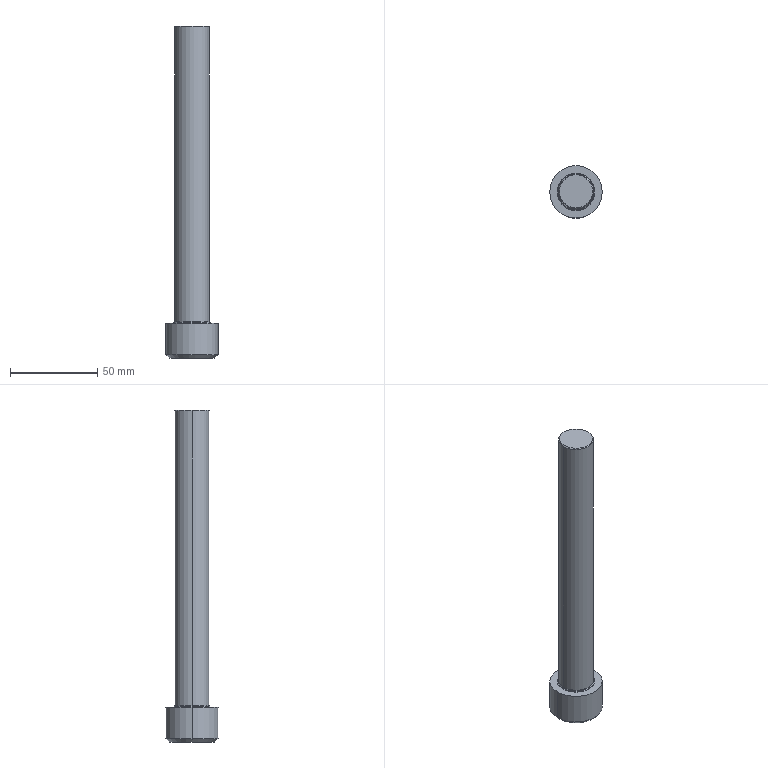Part | Creo | 1 solid | 23 faces | box 30 x 30 x 190 mm | volume 64306 mm3 | plane 9 | cone 6 | cylinder 4 | torus 4 | commonest cylinder face diameters 20 x2 30 x2
STEP:
#1=CARTESIAN_POINT('',(-224.815,189.995,-354.));
#2=VERTEX_POINT('',#1);
#3=CARTESIAN_POINT('',(-219.907,198.495,-354.));
#4=VERTEX_POINT('',#3);
#5=CARTESIAN_POINT('',(-224.815,189.995,-354.));
#6=CARTESIAN_POINT('',(-224.548,190.458,-353.846));
#7=CARTESIAN_POINT('',(-224.012,191.386,-353.574));
#8=CARTESIAN_POINT('',(-223.192,192.806,-353.304));
#9=CARTESIAN_POINT('',(-222.364,194.241,-353.209));
#10=CARTESIAN_POINT('',(-221.532,195.681,-353.304));
#11=CARTESIAN_POINT('',(-220.714,197.099,-353.572));
#12=CARTESIAN_POINT('',(-220.176,198.031,-353.845));
#13=CARTESIAN_POINT('',(-219.907,198.495,-354.));
#14=B_SPLINE_CURVE_WITH_KNOTS('',3,(#5,#6,#7,#8,#9,#10,#11,#12,#13),.UNSPECIFIED.,.F.,.F.,(4,1,1,1,1,1,4),(0.,0.1667,0.3333,0.5,0.6667,0.8333,1.),.UNSPECIFIED.);
#15=EDGE_CURVE('',#2,#4,#14,.T.);
#16=ORIENTED_EDGE('',*,*,#15,.F.);
#17=CARTESIAN_POINT('',(-215.,189.995,-348.333));
#18=VERTEX_POINT('',#17);
#19=CARTESIAN_POINT('',(-215.,189.995,-348.333));
#20=DIRECTION('',(-0.866,0.,-0.5));
#21=VECTOR('',#20,11.333);
#22=LINE('',#19,#21);
#23=EDGE_CURVE('',#18,#2,#22,.T.);
#24=ORIENTED_EDGE('',*,*,#23,.F.);
#25=CARTESIAN_POINT('',(-205.185,189.995,-354.));
#26=VERTEX_POINT('',#25);
#27=CARTESIAN_POINT('',(-215.,189.995,-348.333));
#28=DIRECTION('',(0.866,0.,-0.5));
#29=VECTOR('',#28,11.333);
#30=LINE('',#27,#29);
#31=EDGE_CURVE('',#18,#26,#30,.T.);
#32=ORIENTED_EDGE('',*,*,#31,.T.);
#33=CARTESIAN_POINT('',(-210.093,198.495,-354.));
#34=VERTEX_POINT('',#33);
#35=CARTESIAN_POINT('',(-210.093,198.495,-354.));
#36=CARTESIAN_POINT('',(-209.826,198.033,-353.846));
#37=CARTESIAN_POINT('',(-209.29,197.104,-353.574));
#38=CARTESIAN_POINT('',(-208.47,195.684,-353.304));
#39=CARTESIAN_POINT('',(-207.641,194.25,-353.209));
#40=CARTESIAN_POINT('',(-206.81,192.809,-353.304));
#41=CARTESIAN_POINT('',(-205.991,191.391,-353.572));
#42=CARTESIAN_POINT('',(-205.453,190.46,-353.845));
#43=CARTESIAN_POINT('',(-205.185,189.995,-354.));
#44=B_SPLINE_CURVE_WITH_KNOTS('',3,(#35,#36,#37,#38,#39,#40,#41,#42,#43),.UNSPECIFIED.,.F.,.F.,(4,1,1,1,1,1,4),(0.,0.1667,0.3333,0.5,0.6667,0.8333,1.),.UNSPECIFIED.);
#45=EDGE_CURVE('',#34,#26,#44,.T.);
#46=ORIENTED_EDGE('',*,*,#45,.F.);
#47=CARTESIAN_POINT('',(-219.907,198.495,-354.));
#48=CARTESIAN_POINT('',(-219.376,198.495,-353.847));
#49=CARTESIAN_POINT('',(-218.307,198.495,-353.575));
#50=CARTESIAN_POINT('',(-216.662,198.495,-353.304));
#51=CARTESIAN_POINT('',(-215.002,198.495,-353.209));
#52=CARTESIAN_POINT('',(-213.345,198.495,-353.303));
#53=CARTESIAN_POINT('',(-211.701,198.495,-353.573));
#54=CARTESIAN_POINT('',(-210.627,198.495,-353.846));
#55=CARTESIAN_POINT('',(-210.093,198.495,-354.));
#56=B_SPLINE_CURVE_WITH_KNOTS('',3,(#47,#48,#49,#50,#51,#52,#53,#54,#55),.UNSPECIFIED.,.F.,.F.,(4,1,1,1,1,1,4),(0.,0.1667,0.3333,0.5,0.6667,0.8333,1.),.UNSPECIFIED.);
#57=EDGE_CURVE('',#4,#34,#56,.T.);
#58=ORIENTED_EDGE('',*,*,#57,.F.);
#59=EDGE_LOOP('',(#16,#24,#32,#46,#58));
#60=FACE_OUTER_BOUND('',#59,.F.);
#61=CARTESIAN_POINT('',(-215.,189.995,-351.225));
#62=DIRECTION('',(0.,0.,-1.));
#63=DIRECTION('',(-1.,0.,0.));
#64=AXIS2_PLACEMENT_3D('',#61,#62,#63);
#65=CONICAL_SURFACE('',#64,5.009,60.);
#66=ADVANCED_FACE('',(#60),#65,.F.);
#67=CARTESIAN_POINT('',(-219.907,198.495,-364.));
#68=VERTEX_POINT('',#67);
#69=CARTESIAN_POINT('',(-224.815,189.995,-364.));
#70=VERTEX_POINT('',#69);
#71=CARTESIAN_POINT('',(-219.907,198.495,-364.));
#72=DIRECTION('',(-0.5,-0.866,0.));
#73=VECTOR('',#72,9.815);
#74=LINE('',#71,#73);
#75=EDGE_CURVE('',#68,#70,#74,.T.);
#76=ORIENTED_EDGE('',*,*,#75,.T.);
#77=CARTESIAN_POINT('',(-224.815,189.995,-364.));
#78=DIRECTION('',(0.,0.,1.));
#79=VECTOR('',#78,10.);
#80=LINE('',#77,#79);
#81=EDGE_CURVE('',#70,#2,#80,.T.);
#82=ORIENTED_EDGE('',*,*,#81,.T.);
#83=ORIENTED_EDGE('',*,*,#15,.T.);
#84=CARTESIAN_POINT('',(-219.907,198.495,-364.));
#85=DIRECTION('',(0.,0.,1.));
#86=VECTOR('',#85,10.);
#87=LINE('',#84,#86);
#88=EDGE_CURVE('',#68,#4,#87,.T.);
#89=ORIENTED_EDGE('',*,*,#88,.F.);
#90=EDGE_LOOP('',(#76,#82,#83,#89));
#91=FACE_OUTER_BOUND('',#90,.F.);
#92=CARTESIAN_POINT('',(-219.907,198.495,-354.));
#93=DIRECTION('',(0.866,-0.5,0.));
#94=DIRECTION('',(-0.5,-0.866,0.));
#95=AXIS2_PLACEMENT_3D('',#92,#93,#94);
#96=PLANE('',#95);
#97=ADVANCED_FACE('',(#91),#96,.T.);
#98=CARTESIAN_POINT('',(-228.,189.995,-364.));
#99=VERTEX_POINT('',#98);
#100=CARTESIAN_POINT('',(-202.,189.995,-364.));
#101=VERTEX_POINT('',#100);
#102=CARTESIAN_POINT('',(-215.,189.995,-364.));
#103=DIRECTION('',(0.,0.,-1.));
#104=DIRECTION('',(-1.,0.,0.));
#105=AXIS2_PLACEMENT_3D('',#102,#103,#104);
#106=CIRCLE('',#105,13.);
#107=EDGE_CURVE('',#99,#101,#106,.T.);
#108=ORIENTED_EDGE('',*,*,#107,.F.);
#109=CARTESIAN_POINT('',(-215.,189.995,-364.));
#110=DIRECTION('',(0.,0.,-1.));
#111=DIRECTION('',(1.,0.,0.));
#112=AXIS2_PLACEMENT_3D('',#109,#110,#111);
#113=CIRCLE('',#112,13.);
#114=EDGE_CURVE('',#101,#99,#113,.T.);
#115=ORIENTED_EDGE('',*,*,#114,.F.);
#116=EDGE_LOOP('',(#108,#115));
#117=FACE_OUTER_BOUND('',#116,.F.);
#118=CARTESIAN_POINT('',(-219.907,181.495,-364.));
#119=VERTEX_POINT('',#118);
#120=CARTESIAN_POINT('',(-224.815,189.995,-364.));
#121=DIRECTION('',(0.5,-0.866,0.));
#122=VECTOR('',#121,9.815);
#123=LINE('',#120,#122);
#124=EDGE_CURVE('',#70,#119,#123,.T.);
#125=ORIENTED_EDGE('',*,*,#124,.F.);
#126=ORIENTED_EDGE('',*,*,#75,.F.);
#127=CARTESIAN_POINT('',(-210.093,198.495,-364.));
#128=VERTEX_POINT('',#127);
#129=CARTESIAN_POINT('',(-219.907,198.495,-364.));
#130=DIRECTION('',(1.,0.,0.));
#131=VECTOR('',#130,9.815);
#132=LINE('',#129,#131);
#133=EDGE_CURVE('',#68,#128,#132,.T.);
#134=ORIENTED_EDGE('',*,*,#133,.T.);
#135=CARTESIAN_POINT('',(-205.185,189.995,-364.));
#136=VERTEX_POINT('',#135);
#137=CARTESIAN_POINT('',(-205.185,189.995,-364.));
#138=DIRECTION('',(-0.5,0.866,0.));
#139=VECTOR('',#138,9.815);
#140=LINE('',#137,#139);
#141=EDGE_CURVE('',#136,#128,#140,.T.);
#142=ORIENTED_EDGE('',*,*,#141,.F.);
#143=CARTESIAN_POINT('',(-210.093,181.495,-364.));
#144=VERTEX_POINT('',#143);
#145=CARTESIAN_POINT('',(-210.093,181.495,-364.));
#146=DIRECTION('',(0.5,0.866,0.));
#147=VECTOR('',#146,9.815);
#148=LINE('',#145,#147);
#149=EDGE_CURVE('',#144,#136,#148,.T.);
#150=ORIENTED_EDGE('',*,*,#149,.F.);
#151=CARTESIAN_POINT('',(-210.093,181.495,-364.));
#152=DIRECTION('',(-1.,0.,0.));
#153=VECTOR('',#152,9.815);
#154=LINE('',#151,#153);
#155=EDGE_CURVE('',#144,#119,#154,.T.);
#156=ORIENTED_EDGE('',*,*,#155,.T.);
#157=EDGE_LOOP('',(#125,#126,#134,#142,#150,#156));
#158=FACE_BOUND('',#157,.F.);
#159=CARTESIAN_POINT('',(-215.,189.995,-364.));
#160=DIRECTION('',(0.,0.,-1.));
#161=DIRECTION('',(-1.,0.,0.));
#162=AXIS2_PLACEMENT_3D('',#159,#160,#161);
#163=PLANE('',#162);
#164=ADVANCED_FACE('',(#117,#158),#163,.T.);
#165=CARTESIAN_POINT('',(-230.,189.995,-362.));
#166=VERTEX_POINT('',#165);
#167=CARTESIAN_POINT('',(-200.,189.995,-362.));
#168=VERTEX_POINT('',#167);
#169=CARTESIAN_POINT('',(-215.,189.995,-362.));
#170=DIRECTION('',(0.,0.,-1.));
#171=DIRECTION('',(-1.,0.,0.));
#172=AXIS2_PLACEMENT_3D('',#169,#170,#171);
#173=CIRCLE('',#172,15.);
#174=EDGE_CURVE('',#166,#168,#173,.T.);
#175=ORIENTED_EDGE('',*,*,#174,.F.);
#176=CARTESIAN_POINT('',(-228.,189.995,-364.));
#177=DIRECTION('',(-0.7071,0.,0.7071));
#178=VECTOR('',#177,2.828);
#179=LINE('',#176,#178);
#180=EDGE_CURVE('',#99,#166,#179,.T.);
#181=ORIENTED_EDGE('',*,*,#180,.F.);
#182=ORIENTED_EDGE('',*,*,#107,.T.);
#183=CARTESIAN_POINT('',(-202.,189.995,-364.));
#184=DIRECTION('',(0.7071,0.,0.7071));
#185=VECTOR('',#184,2.828);
#186=LINE('',#183,#185);
#187=EDGE_CURVE('',#101,#168,#186,.T.);
#188=ORIENTED_EDGE('',*,*,#187,.T.);
#189=EDGE_LOOP('',(#175,#181,#182,#188));
#190=FACE_OUTER_BOUND('',#189,.F.);
#191=CARTESIAN_POINT('',(-215.,189.995,-363.));
#192=DIRECTION('',(0.,0.,1.));
#193=DIRECTION('',(1.,0.,0.));
#194=AXIS2_PLACEMENT_3D('',#191,#192,#193);
#195=CONICAL_SURFACE('',#194,14.,45.);
#196=ADVANCED_FACE('',(#190),#195,.T.);
#197=ORIENTED_EDGE('',*,*,#174,.T.);
#198=CARTESIAN_POINT('',(-200.,189.995,-344.));
#199=VERTEX_POINT('',#198);
#200=CARTESIAN_POINT('',(-200.,189.995,-344.));
#201=DIRECTION('',(0.,0.,-1.));
#202=VECTOR('',#201,18.);
#203=LINE('',#200,#202);
#204=EDGE_CURVE('',#199,#168,#203,.T.);
#205=ORIENTED_EDGE('',*,*,#204,.F.);
#206=CARTESIAN_POINT('',(-230.,189.995,-344.));
#207=VERTEX_POINT('',#206);
#208=CARTESIAN_POINT('',(-215.,189.995,-344.));
#209=DIRECTION('',(0.,0.,1.));
#210=DIRECTION('',(1.,0.,0.));
#211=AXIS2_PLACEMENT_3D('',#208,#209,#210);
#212=CIRCLE('',#211,15.);
#213=EDGE_CURVE('',#199,#207,#212,.T.);
#214=ORIENTED_EDGE('',*,*,#213,.T.);
#215=CARTESIAN_POINT('',(-230.,189.995,-344.));
#216=DIRECTION('',(0.,0.,-1.));
#217=VECTOR('',#216,18.);
#218=LINE('',#215,#217);
#219=EDGE_CURVE('',#207,#166,#218,.T.);
#220=ORIENTED_EDGE('',*,*,#219,.T.);
#221=EDGE_LOOP('',(#197,#205,#214,#220));
#222=FACE_OUTER_BOUND('',#221,.F.);
#223=CARTESIAN_POINT('',(-215.,189.995,-344.));
#224=DIRECTION('',(0.,0.,-1.));
#225=DIRECTION('',(-1.,0.,0.));
#226=AXIS2_PLACEMENT_3D('',#223,#224,#225);
#227=CYLINDRICAL_SURFACE('',#226,15.);
#228=ADVANCED_FACE('',(#222),#227,.T.);
#229=CARTESIAN_POINT('',(-215.,189.995,-362.));
#230=DIRECTION('',(0.,0.,-1.));
#231=DIRECTION('',(1.,0.,0.));
#232=AXIS2_PLACEMENT_3D('',#229,#230,#231);
#233=CIRCLE('',#232,15.);
#234=EDGE_CURVE('',#168,#166,#233,.T.);
#235=ORIENTED_EDGE('',*,*,#234,.T.);
#236=ORIENTED_EDGE('',*,*,#219,.F.);
#237=CARTESIAN_POINT('',(-215.,189.995,-344.));
#238=DIRECTION('',(0.,0.,1.));
#239=DIRECTION('',(-1.,0.,0.));
#240=AXIS2_PLACEMENT_3D('',#237,#238,#239);
#241=CIRCLE('',#240,15.);
#242=EDGE_CURVE('',#207,#199,#241,.T.);
#243=ORIENTED_EDGE('',*,*,#242,.T.);
#244=ORIENTED_EDGE('',*,*,#204,.T.);
#245=EDGE_LOOP('',(#235,#236,#243,#244));
#246=FACE_OUTER_BOUND('',#245,.F.);
#247=CARTESIAN_POINT('',(-215.,189.995,-344.));
#248=DIRECTION('',(0.,0.,-1.));
#249=DIRECTION('',(-1.,0.,0.));
#250=AXIS2_PLACEMENT_3D('',#247,#248,#249);
#251=CYLINDRICAL_SURFACE('',#250,15.);
#252=ADVANCED_FACE('',(#246),#251,.T.);
#253=ORIENTED_EDGE('',*,*,#234,.F.);
#254=ORIENTED_EDGE('',*,*,#187,.F.);
#255=ORIENTED_EDGE('',*,*,#114,.T.);
#256=ORIENTED_EDGE('',*,*,#180,.T.);
#257=EDGE_LOOP('',(#253,#254,#255,#256));
#258=FACE_OUTER_BOUND('',#257,.F.);
#259=CARTESIAN_POINT('',(-215.,189.995,-363.));
#260=DIRECTION('',(0.,0.,1.));
#261=DIRECTION('',(1.,0.,0.));
#262=AXIS2_PLACEMENT_3D('',#259,#260,#261);
#263=CONICAL_SURFACE('',#262,14.,45.);
#264=ADVANCED_FACE('',(#258),#263,.T.);
#265=ORIENTED_EDGE('',*,*,#242,.F.);
#266=ORIENTED_EDGE('',*,*,#213,.F.);
#267=EDGE_LOOP('',(#265,#266));
#268=FACE_OUTER_BOUND('',#267,.F.);
#269=CARTESIAN_POINT('',(-225.8,189.995,-344.));
#270=VERTEX_POINT('',#269);
#271=CARTESIAN_POINT('',(-204.2,189.995,-344.));
#272=VERTEX_POINT('',#271);
#273=CARTESIAN_POINT('',(-215.,189.995,-344.));
#274=DIRECTION('',(0.,0.,-1.));
#275=DIRECTION('',(-1.,0.,0.));
#276=AXIS2_PLACEMENT_3D('',#273,#274,#275);
#277=CIRCLE('',#276,10.8);
#278=EDGE_CURVE('',#270,#272,#277,.T.);
#279=ORIENTED_EDGE('',*,*,#278,.F.);
#280=CARTESIAN_POINT('',(-215.,189.995,-344.));
#281=DIRECTION('',(0.,0.,-1.));
#282=DIRECTION('',(1.,0.,0.));
#283=AXIS2_PLACEMENT_3D('',#280,#281,#282);
#284=CIRCLE('',#283,10.8);
#285=EDGE_CURVE('',#272,#270,#284,.T.);
#286=ORIENTED_EDGE('',*,*,#285,.F.);
#287=EDGE_LOOP('',(#279,#286));
#288=FACE_BOUND('',#287,.F.);
#289=CARTESIAN_POINT('',(-215.,189.995,-344.));
#290=DIRECTION('',(0.,0.,-1.));
#291=DIRECTION('',(-1.,0.,0.));
#292=AXIS2_PLACEMENT_3D('',#289,#290,#291);
#293=PLANE('',#292);
#294=ADVANCED_FACE('',(#268,#288),#293,.F.);
#295=ORIENTED_EDGE('',*,*,#278,.T.);
#296=CARTESIAN_POINT('',(-204.766,189.995,-343.766));
#297=VERTEX_POINT('',#296);
#298=CARTESIAN_POINT('',(-204.2,189.995,-343.2));
#299=DIRECTION('',(0.,1.,0.));
#300=DIRECTION('',(0.,0.,-1.));
#301=AXIS2_PLACEMENT_3D('',#298,#299,#300);
#302=CIRCLE('',#301,0.8);
#303=EDGE_CURVE('',#272,#297,#302,.T.);
#304=ORIENTED_EDGE('',*,*,#303,.T.);
#305=CARTESIAN_POINT('',(-225.234,189.995,-343.766));
#306=VERTEX_POINT('',#305);
#307=CARTESIAN_POINT('',(-215.,189.995,-343.766));
#308=DIRECTION('',(0.,0.,-1.));
#309=DIRECTION('',(-1.,0.,0.));
#310=AXIS2_PLACEMENT_3D('',#307,#308,#309);
#311=CIRCLE('',#310,10.234);
#312=EDGE_CURVE('',#306,#297,#311,.T.);
#313=ORIENTED_EDGE('',*,*,#312,.F.);
#314=CARTESIAN_POINT('',(-225.8,189.995,-343.2));
#315=DIRECTION('',(0.,-1.,0.));
#316=DIRECTION('',(0.,0.,-1.));
#317=AXIS2_PLACEMENT_3D('',#314,#315,#316);
#318=CIRCLE('',#317,0.8);
#319=EDGE_CURVE('',#270,#306,#318,.T.);
#320=ORIENTED_EDGE('',*,*,#319,.F.);
#321=EDGE_LOOP('',(#295,#304,#313,#320));
#322=FACE_OUTER_BOUND('',#321,.F.);
#323=CARTESIAN_POINT('',(-215.,189.995,-343.2));
#324=DIRECTION('',(0.,0.,-1.));
#325=DIRECTION('',(-1.,0.,0.));
#326=AXIS2_PLACEMENT_3D('',#323,#324,#325);
#327=TOROIDAL_SURFACE('',#326,10.8,0.8);
#328=ADVANCED_FACE('',(#322),#327,.F.);
#329=ORIENTED_EDGE('',*,*,#285,.T.);
#330=ORIENTED_EDGE('',*,*,#319,.T.);
#331=CARTESIAN_POINT('',(-215.,189.995,-343.766));
#332=DIRECTION('',(0.,0.,-1.));
#333=DIRECTION('',(1.,0.,0.));
#334=AXIS2_PLACEMENT_3D('',#331,#332,#333);
#335=CIRCLE('',#334,10.234);
#336=EDGE_CURVE('',#297,#306,#335,.T.);
#337=ORIENTED_EDGE('',*,*,#336,.F.);
#338=ORIENTED_EDGE('',*,*,#303,.F.);
#339=EDGE_LOOP('',(#329,#330,#337,#338));
#340=FACE_OUTER_BOUND('',#339,.F.);
#341=CARTESIAN_POINT('',(-215.,189.995,-343.2));
#342=DIRECTION('',(0.,0.,-1.));
#343=DIRECTION('',(-1.,0.,0.));
#344=AXIS2_PLACEMENT_3D('',#341,#342,#343);
#345=TOROIDAL_SURFACE('',#344,10.8,0.8);
#346=ADVANCED_FACE('',(#340),#345,.F.);
#347=CARTESIAN_POINT('',(-205.,189.995,-343.2));
#348=VERTEX_POINT('',#347);
#349=CARTESIAN_POINT('',(-225.,189.995,-343.2));
#350=VERTEX_POINT('',#349);
#351=CARTESIAN_POINT('',(-215.,189.995,-343.2));
#352=DIRECTION('',(0.,0.,-1.));
#353=DIRECTION('',(1.,0.,0.));
#354=AXIS2_PLACEMENT_3D('',#351,#352,#353);
#355=CIRCLE('',#354,10.);
#356=EDGE_CURVE('',#348,#350,#355,.T.);
#357=ORIENTED_EDGE('',*,*,#356,.F.);
#358=CARTESIAN_POINT('',(-204.2,189.995,-343.2));
#359=DIRECTION('',(0.,1.,0.));
#360=DIRECTION('',(-0.7071,0.,-0.7071));
#361=AXIS2_PLACEMENT_3D('',#358,#359,#360);
#362=CIRCLE('',#361,0.8);
#363=EDGE_CURVE('',#297,#348,#362,.T.);
#364=ORIENTED_EDGE('',*,*,#363,.F.);
#365=ORIENTED_EDGE('',*,*,#336,.T.);
#366=CARTESIAN_POINT('',(-225.8,189.995,-343.2));
#367=DIRECTION('',(0.,-1.,0.));
#368=DIRECTION('',(0.7071,0.,-0.7071));
#369=AXIS2_PLACEMENT_3D('',#366,#367,#368);
#370=CIRCLE('',#369,0.8);
#371=EDGE_CURVE('',#306,#350,#370,.T.);
#372=ORIENTED_EDGE('',*,*,#371,.T.);
#373=EDGE_LOOP('',(#357,#364,#365,#372));
#374=FACE_OUTER_BOUND('',#373,.F.);
#375=CARTESIAN_POINT('',(-215.,189.995,-343.2));
#376=DIRECTION('',(0.,0.,-1.));
#377=DIRECTION('',(-1.,0.,0.));
#378=AXIS2_PLACEMENT_3D('',#375,#376,#377);
#379=TOROIDAL_SURFACE('',#378,10.8,0.8);
#380=ADVANCED_FACE('',(#374),#379,.F.);
#381=CARTESIAN_POINT('',(-225.,189.995,-174.5));
#382=VERTEX_POINT('',#381);
#383=CARTESIAN_POINT('',(-205.,189.995,-174.5));
#384=VERTEX_POINT('',#383);
#385=CARTESIAN_POINT('',(-215.,189.995,-174.5));
#386=DIRECTION('',(0.,0.,1.));
#387=DIRECTION('',(-1.,0.,0.));
#388=AXIS2_PLACEMENT_3D('',#385,#386,#387);
#389=CIRCLE('',#388,10.);
#390=EDGE_CURVE('',#382,#384,#389,.T.);
#391=ORIENTED_EDGE('',*,*,#390,.T.);
#392=CARTESIAN_POINT('',(-205.,189.995,-174.5));
#393=DIRECTION('',(0.,0.,-1.));
#394=VECTOR('',#393,168.7);
#395=LINE('',#392,#394);
#396=EDGE_CURVE('',#384,#348,#395,.T.);
#397=ORIENTED_EDGE('',*,*,#396,.T.);
#398=ORIENTED_EDGE('',*,*,#356,.T.);
#399=CARTESIAN_POINT('',(-225.,189.995,-174.5));
#400=DIRECTION('',(0.,0.,-1.));
#401=VECTOR('',#400,168.7);
#402=LINE('',#399,#401);
#403=EDGE_CURVE('',#382,#350,#402,.T.);
#404=ORIENTED_EDGE('',*,*,#403,.F.);
#405=EDGE_LOOP('',(#391,#397,#398,#404));
#406=FACE_OUTER_BOUND('',#405,.F.);
#407=CARTESIAN_POINT('',(-215.,189.995,-174.));
#408=DIRECTION('',(0.,0.,-1.));
#409=DIRECTION('',(-1.,0.,0.));
#410=AXIS2_PLACEMENT_3D('',#407,#408,#409);
#411=CYLINDRICAL_SURFACE('',#410,10.);
#412=ADVANCED_FACE('',(#406),#411,.T.);
#413=CARTESIAN_POINT('',(-224.5,189.995,-174.));
#414=VERTEX_POINT('',#413);
#415=CARTESIAN_POINT('',(-205.5,189.995,-174.));
#416=VERTEX_POINT('',#415);
#417=CARTESIAN_POINT('',(-215.,189.995,-174.));
#418=DIRECTION('',(0.,0.,1.));
#419=DIRECTION('',(-1.,0.,0.));
#420=AXIS2_PLACEMENT_3D('',#417,#418,#419);
#421=CIRCLE('',#420,9.5);
#422=EDGE_CURVE('',#414,#416,#421,.T.);
#423=ORIENTED_EDGE('',*,*,#422,.T.);
#424=CARTESIAN_POINT('',(-205.5,189.995,-174.));
#425=DIRECTION('',(0.7071,0.,-0.7071));
#426=VECTOR('',#425,0.7071);
#427=LINE('',#424,#426);
#428=EDGE_CURVE('',#416,#384,#427,.T.);
#429=ORIENTED_EDGE('',*,*,#428,.T.);
#430=ORIENTED_EDGE('',*,*,#390,.F.);
#431=CARTESIAN_POINT('',(-224.5,189.995,-174.));
#432=DIRECTION('',(-0.7071,0.,-0.7071));
#433=VECTOR('',#432,0.7071);
#434=LINE('',#431,#433);
#435=EDGE_CURVE('',#414,#382,#434,.T.);
#436=ORIENTED_EDGE('',*,*,#435,.F.);
#437=EDGE_LOOP('',(#423,#429,#430,#436));
#438=FACE_OUTER_BOUND('',#437,.F.);
#439=CARTESIAN_POINT('',(-215.,189.995,-174.25));
#440=DIRECTION('',(0.,0.,-1.));
#441=DIRECTION('',(-1.,0.,0.));
#442=AXIS2_PLACEMENT_3D('',#439,#440,#441);
#443=CONICAL_SURFACE('',#442,9.75,45.);
#444=ADVANCED_FACE('',(#438),#443,.T.);
#445=ORIENTED_EDGE('',*,*,#422,.F.);
#446=CARTESIAN_POINT('',(-215.,189.995,-174.));
#447=DIRECTION('',(0.,0.,1.));
#448=DIRECTION('',(1.,0.,0.));
#449=AXIS2_PLACEMENT_3D('',#446,#447,#448);
#450=CIRCLE('',#449,9.5);
#451=EDGE_CURVE('',#416,#414,#450,.T.);
#452=ORIENTED_EDGE('',*,*,#451,.F.);
#453=EDGE_LOOP('',(#445,#452));
#454=FACE_OUTER_BOUND('',#453,.F.);
#455=CARTESIAN_POINT('',(-215.,189.995,-174.));
#456=DIRECTION('',(0.,0.,-1.));
#457=DIRECTION('',(-1.,0.,0.));
#458=AXIS2_PLACEMENT_3D('',#455,#456,#457);
#459=PLANE('',#458);
#460=ADVANCED_FACE('',(#454),#459,.F.);
#461=ORIENTED_EDGE('',*,*,#451,.T.);
#462=ORIENTED_EDGE('',*,*,#435,.T.);
#463=CARTESIAN_POINT('',(-215.,189.995,-174.5));
#464=DIRECTION('',(0.,0.,1.));
#465=DIRECTION('',(1.,0.,0.));
#466=AXIS2_PLACEMENT_3D('',#463,#464,#465);
#467=CIRCLE('',#466,10.);
#468=EDGE_CURVE('',#384,#382,#467,.T.);
#469=ORIENTED_EDGE('',*,*,#468,.F.);
#470=ORIENTED_EDGE('',*,*,#428,.F.);
#471=EDGE_LOOP('',(#461,#462,#469,#470));
#472=FACE_OUTER_BOUND('',#471,.F.);
#473=CARTESIAN_POINT('',(-215.,189.995,-174.25));
#474=DIRECTION('',(0.,0.,-1.));
#475=DIRECTION('',(-1.,0.,0.));
#476=AXIS2_PLACEMENT_3D('',#473,#474,#475);
#477=CONICAL_SURFACE('',#476,9.75,45.);
#478=ADVANCED_FACE('',(#472),#477,.T.);
#479=ORIENTED_EDGE('',*,*,#468,.T.);
#480=ORIENTED_EDGE('',*,*,#403,.T.);
#481=CARTESIAN_POINT('',(-215.,189.995,-343.2));
#482=DIRECTION('',(0.,0.,-1.));
#483=DIRECTION('',(-1.,0.,0.));
#484=AXIS2_PLACEMENT_3D('',#481,#482,#483);
#485=CIRCLE('',#484,10.);
#486=EDGE_CURVE('',#350,#348,#485,.T.);
#487=ORIENTED_EDGE('',*,*,#486,.T.);
#488=ORIENTED_EDGE('',*,*,#396,.F.);
#489=EDGE_LOOP('',(#479,#480,#487,#488));
#490=FACE_OUTER_BOUND('',#489,.F.);
#491=CARTESIAN_POINT('',(-215.,189.995,-174.));
#492=DIRECTION('',(0.,0.,-1.));
#493=DIRECTION('',(-1.,0.,0.));
#494=AXIS2_PLACEMENT_3D('',#491,#492,#493);
#495=CYLINDRICAL_SURFACE('',#494,10.);
#496=ADVANCED_FACE('',(#490),#495,.T.);
#497=ORIENTED_EDGE('',*,*,#486,.F.);
#498=ORIENTED_EDGE('',*,*,#371,.F.);
#499=ORIENTED_EDGE('',*,*,#312,.T.);
#500=ORIENTED_EDGE('',*,*,#363,.T.);
#501=EDGE_LOOP('',(#497,#498,#499,#500));
#502=FACE_OUTER_BOUND('',#501,.F.);
#503=CARTESIAN_POINT('',(-215.,189.995,-343.2));
#504=DIRECTION('',(0.,0.,-1.));
#505=DIRECTION('',(-1.,0.,0.));
#506=AXIS2_PLACEMENT_3D('',#503,#504,#505);
#507=TOROIDAL_SURFACE('',#506,10.8,0.8);
#508=ADVANCED_FACE('',(#502),#507,.F.);
#509=ORIENTED_EDGE('',*,*,#124,.T.);
#510=CARTESIAN_POINT('',(-219.907,181.495,-354.));
#511=VERTEX_POINT('',#510);
#512=CARTESIAN_POINT('',(-219.907,181.495,-364.));
#513=DIRECTION('',(0.,0.,1.));
#514=VECTOR('',#513,10.);
#515=LINE('',#512,#514);
#516=EDGE_CURVE('',#119,#511,#515,.T.);
#517=ORIENTED_EDGE('',*,*,#516,.T.);
#518=CARTESIAN_POINT('',(-219.907,181.495,-354.));
#519=CARTESIAN_POINT('',(-220.174,181.958,-353.846));
#520=CARTESIAN_POINT('',(-220.71,182.886,-353.574));
#521=CARTESIAN_POINT('',(-221.53,184.306,-353.304));
#522=CARTESIAN_POINT('',(-222.359,185.741,-353.209));
#523=CARTESIAN_POINT('',(-223.19,187.181,-353.304));
#524=CARTESIAN_POINT('',(-224.009,188.599,-353.572));
#525=CARTESIAN_POINT('',(-224.547,189.531,-353.845));
#526=CARTESIAN_POINT('',(-224.815,189.995,-354.));
#527=B_SPLINE_CURVE_WITH_KNOTS('',3,(#518,#519,#520,#521,#522,#523,#524,#525,#526),.UNSPECIFIED.,.F.,.F.,(4,1,1,1,1,1,4),(0.,0.1667,0.3333,0.5,0.6667,0.8333,1.),.UNSPECIFIED.);
#528=EDGE_CURVE('',#511,#2,#527,.T.);
#529=ORIENTED_EDGE('',*,*,#528,.T.);
#530=ORIENTED_EDGE('',*,*,#81,.F.);
#531=EDGE_LOOP('',(#509,#517,#529,#530));
#532=FACE_OUTER_BOUND('',#531,.F.);
#533=CARTESIAN_POINT('',(-224.815,189.995,-354.));
#534=DIRECTION('',(0.866,0.5,0.));
#535=DIRECTION('',(0.5,-0.866,0.));
#536=AXIS2_PLACEMENT_3D('',#533,#534,#535);
#537=PLANE('',#536);
#538=ADVANCED_FACE('',(#532),#537,.T.);
#539=ORIENTED_EDGE('',*,*,#155,.F.);
#540=CARTESIAN_POINT('',(-210.093,181.495,-354.));
#541=VERTEX_POINT('',#540);
#542=CARTESIAN_POINT('',(-210.093,181.495,-364.));
#543=DIRECTION('',(0.,0.,1.));
#544=VECTOR('',#543,10.);
#545=LINE('',#542,#544);
#546=EDGE_CURVE('',#144,#541,#545,.T.);
#547=ORIENTED_EDGE('',*,*,#546,.T.);
#548=CARTESIAN_POINT('',(-210.093,181.495,-354.));
#549=CARTESIAN_POINT('',(-210.627,181.495,-353.846));
#550=CARTESIAN_POINT('',(-211.701,181.495,-353.573));
#551=CARTESIAN_POINT('',(-213.345,181.495,-353.303));
#552=CARTESIAN_POINT('',(-215.002,181.495,-353.209));
#553=CARTESIAN_POINT('',(-216.662,181.495,-353.304));
#554=CARTESIAN_POINT('',(-218.307,181.495,-353.575));
#555=CARTESIAN_POINT('',(-219.376,181.495,-353.847));
#556=CARTESIAN_POINT('',(-219.907,181.495,-354.));
#557=B_SPLINE_CURVE_WITH_KNOTS('',3,(#548,#549,#550,#551,#552,#553,#554,#555,#556),.UNSPECIFIED.,.F.,.F.,(4,1,1,1,1,1,4),(0.,0.1667,0.3333,0.5,0.6667,0.8333,1.),.UNSPECIFIED.);
#558=EDGE_CURVE('',#541,#511,#557,.T.);
#559=ORIENTED_EDGE('',*,*,#558,.T.);
#560=ORIENTED_EDGE('',*,*,#516,.F.);
#561=EDGE_LOOP('',(#539,#547,#559,#560));
#562=FACE_OUTER_BOUND('',#561,.F.);
#563=CARTESIAN_POINT('',(-219.907,181.495,-354.));
#564=DIRECTION('',(0.,1.,0.));
#565=DIRECTION('',(0.,0.,-1.));
#566=AXIS2_PLACEMENT_3D('',#563,#564,#565);
#567=PLANE('',#566);
#568=ADVANCED_FACE('',(#562),#567,.T.);
#569=ORIENTED_EDGE('',*,*,#149,.T.);
#570=CARTESIAN_POINT('',(-205.185,189.995,-364.));
#571=DIRECTION('',(0.,0.,1.));
#572=VECTOR('',#571,10.);
#573=LINE('',#570,#572);
#574=EDGE_CURVE('',#136,#26,#573,.T.);
#575=ORIENTED_EDGE('',*,*,#574,.T.);
#576=CARTESIAN_POINT('',(-205.185,189.995,-354.));
#577=CARTESIAN_POINT('',(-205.453,189.531,-353.845));
#578=CARTESIAN_POINT('',(-205.991,188.599,-353.572));
#579=CARTESIAN_POINT('',(-206.81,187.181,-353.304));
#580=CARTESIAN_POINT('',(-207.641,185.741,-353.209));
#581=CARTESIAN_POINT('',(-208.47,184.306,-353.304));
#582=CARTESIAN_POINT('',(-209.289,182.886,-353.574));
#583=CARTESIAN_POINT('',(-209.826,181.958,-353.846));
#584=CARTESIAN_POINT('',(-210.093,181.495,-354.));
#585=B_SPLINE_CURVE_WITH_KNOTS('',3,(#576,#577,#578,#579,#580,#581,#582,#583,#584),.UNSPECIFIED.,.F.,.F.,(4,1,1,1,1,1,4),(0.,0.1667,0.3333,0.5,0.6667,0.8333,1.),.UNSPECIFIED.);
#586=EDGE_CURVE('',#26,#541,#585,.T.);
#587=ORIENTED_EDGE('',*,*,#586,.T.);
#588=ORIENTED_EDGE('',*,*,#546,.F.);
#589=EDGE_LOOP('',(#569,#575,#587,#588));
#590=FACE_OUTER_BOUND('',#589,.F.);
#591=CARTESIAN_POINT('',(-210.093,181.495,-354.));
#592=DIRECTION('',(-0.866,0.5,0.));
#593=DIRECTION('',(0.5,0.866,0.));
#594=AXIS2_PLACEMENT_3D('',#591,#592,#593);
#595=PLANE('',#594);
#596=ADVANCED_FACE('',(#590),#595,.T.);
#597=ORIENTED_EDGE('',*,*,#141,.T.);
#598=CARTESIAN_POINT('',(-210.093,198.495,-364.));
#599=DIRECTION('',(0.,0.,1.));
#600=VECTOR('',#599,10.);
#601=LINE('',#598,#600);
#602=EDGE_CURVE('',#128,#34,#601,.T.);
#603=ORIENTED_EDGE('',*,*,#602,.T.);
#604=ORIENTED_EDGE('',*,*,#45,.T.);
#605=ORIENTED_EDGE('',*,*,#574,.F.);
#606=EDGE_LOOP('',(#597,#603,#604,#605));
#607=FACE_OUTER_BOUND('',#606,.F.);
#608=CARTESIAN_POINT('',(-205.185,189.995,-354.));
#609=DIRECTION('',(-0.866,-0.5,0.));
#610=DIRECTION('',(-0.5,0.866,0.));
#611=AXIS2_PLACEMENT_3D('',#608,#609,#610);
#612=PLANE('',#611);
#613=ADVANCED_FACE('',(#607),#612,.T.);
#614=ORIENTED_EDGE('',*,*,#133,.F.);
#615=ORIENTED_EDGE('',*,*,#88,.T.);
#616=ORIENTED_EDGE('',*,*,#57,.T.);
#617=ORIENTED_EDGE('',*,*,#602,.F.);
#618=EDGE_LOOP('',(#614,#615,#616,#617));
#619=FACE_OUTER_BOUND('',#618,.F.);
#620=CARTESIAN_POINT('',(-210.093,198.495,-354.));
#621=DIRECTION('',(0.,-1.,0.));
#622=DIRECTION('',(0.,0.,1.));
#623=AXIS2_PLACEMENT_3D('',#620,#621,#622);
#624=PLANE('',#623);
#625=ADVANCED_FACE('',(#619),#624,.T.);
#626=ORIENTED_EDGE('',*,*,#586,.F.);
#627=ORIENTED_EDGE('',*,*,#31,.F.);
#628=ORIENTED_EDGE('',*,*,#23,.T.);
#629=ORIENTED_EDGE('',*,*,#528,.F.);
#630=ORIENTED_EDGE('',*,*,#558,.F.);
#631=EDGE_LOOP('',(#626,#627,#628,#629,#630));
#632=FACE_OUTER_BOUND('',#631,.F.);
#633=CARTESIAN_POINT('',(-215.,189.995,-351.225));
#634=DIRECTION('',(0.,0.,-1.));
#635=DIRECTION('',(-1.,0.,0.));
#636=AXIS2_PLACEMENT_3D('',#633,#634,#635);
#637=CONICAL_SURFACE('',#636,5.009,60.);
#638=ADVANCED_FACE('',(#632),#637,.F.);
#639=CLOSED_SHELL('',(#66,#97,#164,#196,#228,#252,#264,#294,#328,#346,#380,#412,#444,#460,#478,#496,#508,#538,#568,#596,#613,#625,#638));
#640=MANIFOLD_SOLID_BREP('',#639);
#641=(LENGTH_UNIT()NAMED_UNIT(*)SI_UNIT(.MILLI.,.METRE.));
#642=UNCERTAINTY_MEASURE_WITH_UNIT(LENGTH_MEASURE(0.01947),#641,'','');
#643=(NAMED_UNIT(*)PLANE_ANGLE_UNIT()SI_UNIT($,.RADIAN.));
#644=PLANE_ANGLE_MEASURE_WITH_UNIT(PLANE_ANGLE_MEASURE(0.01745),#643);
#645=(CONVERSION_BASED_UNIT('DEGREE',#644)NAMED_UNIT(*)PLANE_ANGLE_UNIT());
#646=(NAMED_UNIT(*)SI_UNIT($,.STERADIAN.)SOLID_ANGLE_UNIT());
#647=(GEOMETRIC_REPRESENTATION_CONTEXT(3)GLOBAL_UNCERTAINTY_ASSIGNED_CONTEXT((#642))GLOBAL_UNIT_ASSIGNED_CONTEXT((#641,#645,#646))REPRESENTATION_CONTEXT('',''));
#648=ADVANCED_BREP_SHAPE_REPRESENTATION('',(#640),#647);